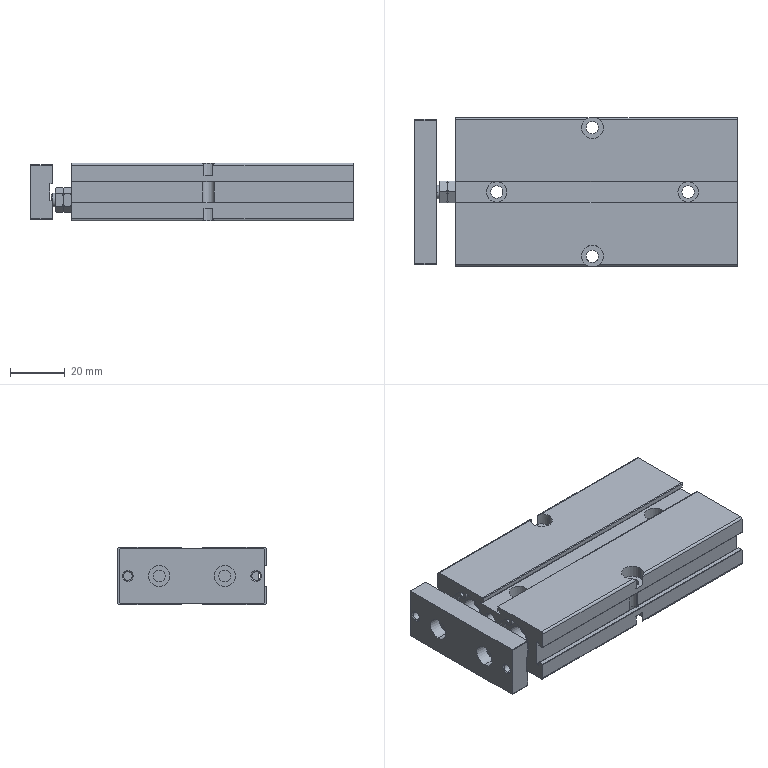Part | SolidWorks | 2 solids | 289 faces | box 118 x 54.3 x 21.2 mm | volume 85401 mm3 | cylinder 140 | plane 97 | cone 52 | commonest cylinder face diameters 0.4 x30 1.52 x16 8 x16 3.5 x12 16 x12 1.6 x8